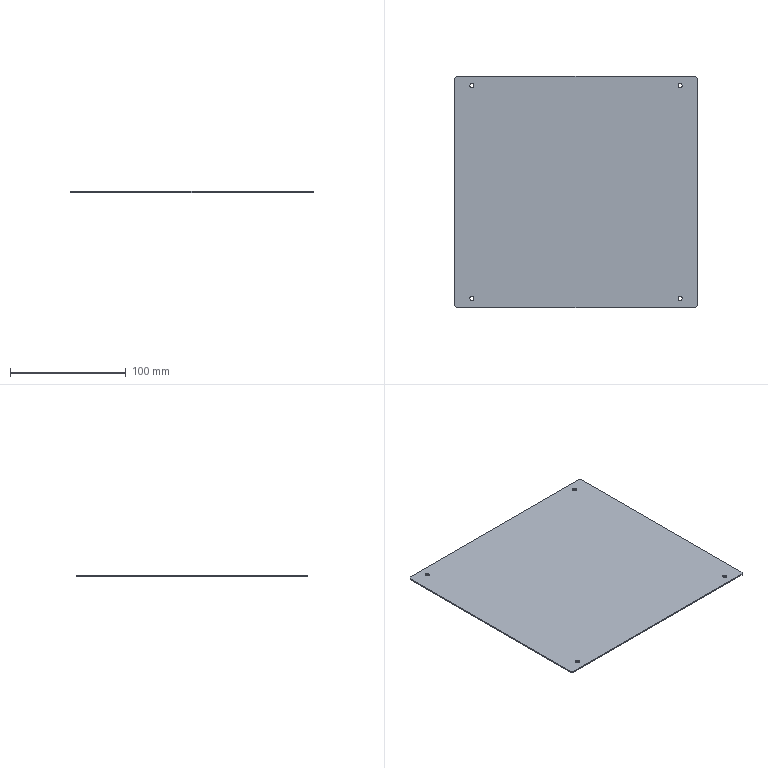Part | NX | 1 solid | 18 faces | box 210 x 200 x 1 mm | volume 41954 mm3 | plane 10 | cylinder 8 | commonest cylinder face diameters 3.5 x8
STEP:
#1=CARTESIAN_POINT('',(-105.,-98.,-0.5));
#2=VERTEX_POINT('',#1);
#3=CARTESIAN_POINT('',(-105.,98.,-0.5));
#4=VERTEX_POINT('',#3);
#5=CARTESIAN_POINT('',(-105.,-98.,-0.5));
#6=DIRECTION('',(0.,1.,0.));
#7=VECTOR('',#6,1000.);
#8=LINE('',#5,#7);
#9=EDGE_CURVE('',#2,#4,#8,.T.);
#10=ORIENTED_EDGE('',*,*,#9,.T.);
#11=CARTESIAN_POINT('',(-103.,100.,-0.5));
#12=VERTEX_POINT('',#11);
#13=CARTESIAN_POINT('',(-103.,100.,-0.5));
#14=DIRECTION('',(-0.7071,-0.7071,0.));
#15=VECTOR('',#14,1000.);
#16=LINE('',#13,#15);
#17=EDGE_CURVE('',#12,#4,#16,.T.);
#18=ORIENTED_EDGE('',*,*,#17,.F.);
#19=CARTESIAN_POINT('',(103.,100.,-0.5));
#20=VERTEX_POINT('',#19);
#21=CARTESIAN_POINT('',(-103.,100.,-0.5));
#22=DIRECTION('',(1.,0.,0.));
#23=VECTOR('',#22,1000.);
#24=LINE('',#21,#23);
#25=EDGE_CURVE('',#12,#20,#24,.T.);
#26=ORIENTED_EDGE('',*,*,#25,.T.);
#27=CARTESIAN_POINT('',(105.,98.,-0.5));
#28=VERTEX_POINT('',#27);
#29=CARTESIAN_POINT('',(105.,98.,-0.5));
#30=DIRECTION('',(-0.7071,0.7071,0.));
#31=VECTOR('',#30,1000.);
#32=LINE('',#29,#31);
#33=EDGE_CURVE('',#28,#20,#32,.T.);
#34=ORIENTED_EDGE('',*,*,#33,.F.);
#35=CARTESIAN_POINT('',(105.,-98.,-0.5));
#36=VERTEX_POINT('',#35);
#37=CARTESIAN_POINT('',(105.,98.,-0.5));
#38=DIRECTION('',(0.,-1.,0.));
#39=VECTOR('',#38,1000.);
#40=LINE('',#37,#39);
#41=EDGE_CURVE('',#28,#36,#40,.T.);
#42=ORIENTED_EDGE('',*,*,#41,.T.);
#43=CARTESIAN_POINT('',(103.,-100.,-0.5));
#44=VERTEX_POINT('',#43);
#45=CARTESIAN_POINT('',(103.,-100.,-0.5));
#46=DIRECTION('',(0.7071,0.7071,0.));
#47=VECTOR('',#46,1000.);
#48=LINE('',#45,#47);
#49=EDGE_CURVE('',#44,#36,#48,.T.);
#50=ORIENTED_EDGE('',*,*,#49,.F.);
#51=CARTESIAN_POINT('',(-103.,-100.,-0.5));
#52=VERTEX_POINT('',#51);
#53=CARTESIAN_POINT('',(103.,-100.,-0.5));
#54=DIRECTION('',(-1.,0.,0.));
#55=VECTOR('',#54,1000.);
#56=LINE('',#53,#55);
#57=EDGE_CURVE('',#44,#52,#56,.T.);
#58=ORIENTED_EDGE('',*,*,#57,.T.);
#59=CARTESIAN_POINT('',(-105.,-98.,-0.5));
#60=DIRECTION('',(0.7071,-0.7071,0.));
#61=VECTOR('',#60,1000.);
#62=LINE('',#59,#61);
#63=EDGE_CURVE('',#2,#52,#62,.T.);
#64=ORIENTED_EDGE('',*,*,#63,.F.);
#65=EDGE_LOOP('',(#10,#18,#26,#34,#42,#50,#58,#64));
#66=FACE_BOUND('',#65,.T.);
#67=CARTESIAN_POINT('',(-88.25,-92.,-0.5));
#68=VERTEX_POINT('',#67);
#69=CARTESIAN_POINT('',(-91.75,-92.,-0.5));
#70=VERTEX_POINT('',#69);
#71=CARTESIAN_POINT('',(-90.,-92.,-0.5));
#72=DIRECTION('',(0.,0.,-1.));
#73=DIRECTION('',(1.,0.,0.));
#74=AXIS2_PLACEMENT_3D('',#71,#72,#73);
#75=CIRCLE('',#74,1.75);
#76=EDGE_CURVE('',#68,#70,#75,.T.);
#77=ORIENTED_EDGE('',*,*,#76,.F.);
#78=CARTESIAN_POINT('',(-90.,-92.,-0.5));
#79=DIRECTION('',(0.,0.,-1.));
#80=DIRECTION('',(1.,0.,0.));
#81=AXIS2_PLACEMENT_3D('',#78,#79,#80);
#82=CIRCLE('',#81,1.75);
#83=EDGE_CURVE('',#70,#68,#82,.T.);
#84=ORIENTED_EDGE('',*,*,#83,.F.);
#85=EDGE_LOOP('',(#77,#84));
#86=FACE_BOUND('',#85,.T.);
#87=CARTESIAN_POINT('',(91.75,-92.,-0.5));
#88=VERTEX_POINT('',#87);
#89=CARTESIAN_POINT('',(88.25,-92.,-0.5));
#90=VERTEX_POINT('',#89);
#91=CARTESIAN_POINT('',(90.,-92.,-0.5));
#92=DIRECTION('',(0.,0.,-1.));
#93=DIRECTION('',(1.,0.,0.));
#94=AXIS2_PLACEMENT_3D('',#91,#92,#93);
#95=CIRCLE('',#94,1.75);
#96=EDGE_CURVE('',#88,#90,#95,.T.);
#97=ORIENTED_EDGE('',*,*,#96,.F.);
#98=CARTESIAN_POINT('',(90.,-92.,-0.5));
#99=DIRECTION('',(0.,0.,-1.));
#100=DIRECTION('',(1.,0.,0.));
#101=AXIS2_PLACEMENT_3D('',#98,#99,#100);
#102=CIRCLE('',#101,1.75);
#103=EDGE_CURVE('',#90,#88,#102,.T.);
#104=ORIENTED_EDGE('',*,*,#103,.F.);
#105=EDGE_LOOP('',(#97,#104));
#106=FACE_BOUND('',#105,.T.);
#107=CARTESIAN_POINT('',(-88.25,92.,-0.5));
#108=VERTEX_POINT('',#107);
#109=CARTESIAN_POINT('',(-91.75,92.,-0.5));
#110=VERTEX_POINT('',#109);
#111=CARTESIAN_POINT('',(-90.,92.,-0.5));
#112=DIRECTION('',(0.,0.,-1.));
#113=DIRECTION('',(1.,0.,0.));
#114=AXIS2_PLACEMENT_3D('',#111,#112,#113);
#115=CIRCLE('',#114,1.75);
#116=EDGE_CURVE('',#108,#110,#115,.T.);
#117=ORIENTED_EDGE('',*,*,#116,.F.);
#118=CARTESIAN_POINT('',(-90.,92.,-0.5));
#119=DIRECTION('',(0.,0.,-1.));
#120=DIRECTION('',(1.,0.,0.));
#121=AXIS2_PLACEMENT_3D('',#118,#119,#120);
#122=CIRCLE('',#121,1.75);
#123=EDGE_CURVE('',#110,#108,#122,.T.);
#124=ORIENTED_EDGE('',*,*,#123,.F.);
#125=EDGE_LOOP('',(#117,#124));
#126=FACE_BOUND('',#125,.T.);
#127=CARTESIAN_POINT('',(88.25,92.,-0.5));
#128=VERTEX_POINT('',#127);
#129=CARTESIAN_POINT('',(91.75,92.,-0.5));
#130=VERTEX_POINT('',#129);
#131=CARTESIAN_POINT('',(90.,92.,-0.5));
#132=DIRECTION('',(0.,0.,-1.));
#133=DIRECTION('',(1.,0.,0.));
#134=AXIS2_PLACEMENT_3D('',#131,#132,#133);
#135=CIRCLE('',#134,1.75);
#136=EDGE_CURVE('',#128,#130,#135,.T.);
#137=ORIENTED_EDGE('',*,*,#136,.F.);
#138=CARTESIAN_POINT('',(90.,92.,-0.5));
#139=DIRECTION('',(0.,0.,-1.));
#140=DIRECTION('',(1.,0.,0.));
#141=AXIS2_PLACEMENT_3D('',#138,#139,#140);
#142=CIRCLE('',#141,1.75);
#143=EDGE_CURVE('',#130,#128,#142,.T.);
#144=ORIENTED_EDGE('',*,*,#143,.F.);
#145=EDGE_LOOP('',(#137,#144));
#146=FACE_BOUND('',#145,.T.);
#147=CARTESIAN_POINT('',(0.,0.,-0.5));
#148=DIRECTION('',(0.,0.,1.));
#149=DIRECTION('',(1.,0.,0.));
#150=AXIS2_PLACEMENT_3D('',#147,#148,#149);
#151=PLANE('',#150);
#152=ADVANCED_FACE('',(#66,#86,#106,#126,#146),#151,.F.);
#153=ORIENTED_EDGE('',*,*,#9,.F.);
#154=CARTESIAN_POINT('',(-105.,-98.,0.5));
#155=VERTEX_POINT('',#154);
#156=CARTESIAN_POINT('',(-105.,-98.,0.5));
#157=DIRECTION('',(0.,0.,-1.));
#158=VECTOR('',#157,1000.);
#159=LINE('',#156,#158);
#160=EDGE_CURVE('',#155,#2,#159,.T.);
#161=ORIENTED_EDGE('',*,*,#160,.F.);
#162=CARTESIAN_POINT('',(-105.,98.,0.5));
#163=VERTEX_POINT('',#162);
#164=CARTESIAN_POINT('',(-105.,-98.,0.5));
#165=DIRECTION('',(0.,1.,0.));
#166=VECTOR('',#165,1000.);
#167=LINE('',#164,#166);
#168=EDGE_CURVE('',#155,#163,#167,.T.);
#169=ORIENTED_EDGE('',*,*,#168,.T.);
#170=CARTESIAN_POINT('',(-105.,98.,0.5));
#171=DIRECTION('',(0.,0.,-1.));
#172=VECTOR('',#171,1000.);
#173=LINE('',#170,#172);
#174=EDGE_CURVE('',#163,#4,#173,.T.);
#175=ORIENTED_EDGE('',*,*,#174,.T.);
#176=EDGE_LOOP('',(#153,#161,#169,#175));
#177=FACE_BOUND('',#176,.T.);
#178=CARTESIAN_POINT('',(-105.,100.,-0.5));
#179=DIRECTION('',(-1.,0.,0.));
#180=DIRECTION('',(0.,0.,1.));
#181=AXIS2_PLACEMENT_3D('',#178,#179,#180);
#182=PLANE('',#181);
#183=ADVANCED_FACE('',(#177),#182,.T.);
#184=ORIENTED_EDGE('',*,*,#174,.F.);
#185=CARTESIAN_POINT('',(-103.,100.,0.5));
#186=VERTEX_POINT('',#185);
#187=CARTESIAN_POINT('',(-105.,98.,0.5));
#188=DIRECTION('',(0.7071,0.7071,0.));
#189=VECTOR('',#188,1000.);
#190=LINE('',#187,#189);
#191=EDGE_CURVE('',#163,#186,#190,.T.);
#192=ORIENTED_EDGE('',*,*,#191,.T.);
#193=CARTESIAN_POINT('',(-103.,100.,0.5));
#194=DIRECTION('',(0.,0.,-1.));
#195=VECTOR('',#194,1000.);
#196=LINE('',#193,#195);
#197=EDGE_CURVE('',#186,#12,#196,.T.);
#198=ORIENTED_EDGE('',*,*,#197,.T.);
#199=ORIENTED_EDGE('',*,*,#17,.T.);
#200=EDGE_LOOP('',(#184,#192,#198,#199));
#201=FACE_BOUND('',#200,.T.);
#202=CARTESIAN_POINT('',(-105.,98.,-0.5));
#203=DIRECTION('',(-0.7071,0.7071,0.));
#204=DIRECTION('',(0.,0.,1.));
#205=AXIS2_PLACEMENT_3D('',#202,#203,#204);
#206=PLANE('',#205);
#207=ADVANCED_FACE('',(#201),#206,.T.);
#208=ORIENTED_EDGE('',*,*,#25,.F.);
#209=ORIENTED_EDGE('',*,*,#197,.F.);
#210=CARTESIAN_POINT('',(103.,100.,0.5));
#211=VERTEX_POINT('',#210);
#212=CARTESIAN_POINT('',(-103.,100.,0.5));
#213=DIRECTION('',(1.,0.,0.));
#214=VECTOR('',#213,1000.);
#215=LINE('',#212,#214);
#216=EDGE_CURVE('',#186,#211,#215,.T.);
#217=ORIENTED_EDGE('',*,*,#216,.T.);
#218=CARTESIAN_POINT('',(103.,100.,0.5));
#219=DIRECTION('',(0.,0.,-1.));
#220=VECTOR('',#219,1000.);
#221=LINE('',#218,#220);
#222=EDGE_CURVE('',#211,#20,#221,.T.);
#223=ORIENTED_EDGE('',*,*,#222,.T.);
#224=EDGE_LOOP('',(#208,#209,#217,#223));
#225=FACE_BOUND('',#224,.T.);
#226=CARTESIAN_POINT('',(105.,100.,-0.5));
#227=DIRECTION('',(0.,1.,0.));
#228=DIRECTION('',(1.,0.,0.));
#229=AXIS2_PLACEMENT_3D('',#226,#227,#228);
#230=PLANE('',#229);
#231=ADVANCED_FACE('',(#225),#230,.T.);
#232=ORIENTED_EDGE('',*,*,#222,.F.);
#233=CARTESIAN_POINT('',(105.,98.,0.5));
#234=VERTEX_POINT('',#233);
#235=CARTESIAN_POINT('',(103.,100.,0.5));
#236=DIRECTION('',(0.7071,-0.7071,0.));
#237=VECTOR('',#236,1000.);
#238=LINE('',#235,#237);
#239=EDGE_CURVE('',#211,#234,#238,.T.);
#240=ORIENTED_EDGE('',*,*,#239,.T.);
#241=CARTESIAN_POINT('',(105.,98.,0.5));
#242=DIRECTION('',(0.,0.,-1.));
#243=VECTOR('',#242,1000.);
#244=LINE('',#241,#243);
#245=EDGE_CURVE('',#234,#28,#244,.T.);
#246=ORIENTED_EDGE('',*,*,#245,.T.);
#247=ORIENTED_EDGE('',*,*,#33,.T.);
#248=EDGE_LOOP('',(#232,#240,#246,#247));
#249=FACE_BOUND('',#248,.T.);
#250=CARTESIAN_POINT('',(103.,100.,-0.5));
#251=DIRECTION('',(0.7071,0.7071,0.));
#252=DIRECTION('',(0.,0.,-1.));
#253=AXIS2_PLACEMENT_3D('',#250,#251,#252);
#254=PLANE('',#253);
#255=ADVANCED_FACE('',(#249),#254,.T.);
#256=ORIENTED_EDGE('',*,*,#41,.F.);
#257=ORIENTED_EDGE('',*,*,#245,.F.);
#258=CARTESIAN_POINT('',(105.,-98.,0.5));
#259=VERTEX_POINT('',#258);
#260=CARTESIAN_POINT('',(105.,98.,0.5));
#261=DIRECTION('',(0.,-1.,0.));
#262=VECTOR('',#261,1000.);
#263=LINE('',#260,#262);
#264=EDGE_CURVE('',#234,#259,#263,.T.);
#265=ORIENTED_EDGE('',*,*,#264,.T.);
#266=CARTESIAN_POINT('',(105.,-98.,0.5));
#267=DIRECTION('',(0.,0.,-1.));
#268=VECTOR('',#267,1000.);
#269=LINE('',#266,#268);
#270=EDGE_CURVE('',#259,#36,#269,.T.);
#271=ORIENTED_EDGE('',*,*,#270,.T.);
#272=EDGE_LOOP('',(#256,#257,#265,#271));
#273=FACE_BOUND('',#272,.T.);
#274=CARTESIAN_POINT('',(105.,-100.,-0.5));
#275=DIRECTION('',(1.,0.,0.));
#276=DIRECTION('',(0.,1.,0.));
#277=AXIS2_PLACEMENT_3D('',#274,#275,#276);
#278=PLANE('',#277);
#279=ADVANCED_FACE('',(#273),#278,.T.);
#280=ORIENTED_EDGE('',*,*,#270,.F.);
#281=CARTESIAN_POINT('',(103.,-100.,0.5));
#282=VERTEX_POINT('',#281);
#283=CARTESIAN_POINT('',(105.,-98.,0.5));
#284=DIRECTION('',(-0.7071,-0.7071,0.));
#285=VECTOR('',#284,1000.);
#286=LINE('',#283,#285);
#287=EDGE_CURVE('',#259,#282,#286,.T.);
#288=ORIENTED_EDGE('',*,*,#287,.T.);
#289=CARTESIAN_POINT('',(103.,-100.,0.5));
#290=DIRECTION('',(0.,0.,-1.));
#291=VECTOR('',#290,1000.);
#292=LINE('',#289,#291);
#293=EDGE_CURVE('',#282,#44,#292,.T.);
#294=ORIENTED_EDGE('',*,*,#293,.T.);
#295=ORIENTED_EDGE('',*,*,#49,.T.);
#296=EDGE_LOOP('',(#280,#288,#294,#295));
#297=FACE_BOUND('',#296,.T.);
#298=CARTESIAN_POINT('',(105.,-98.,-0.5));
#299=DIRECTION('',(0.7071,-0.7071,0.));
#300=DIRECTION('',(0.,0.,-1.));
#301=AXIS2_PLACEMENT_3D('',#298,#299,#300);
#302=PLANE('',#301);
#303=ADVANCED_FACE('',(#297),#302,.T.);
#304=ORIENTED_EDGE('',*,*,#57,.F.);
#305=ORIENTED_EDGE('',*,*,#293,.F.);
#306=CARTESIAN_POINT('',(-103.,-100.,0.5));
#307=VERTEX_POINT('',#306);
#308=CARTESIAN_POINT('',(103.,-100.,0.5));
#309=DIRECTION('',(-1.,0.,0.));
#310=VECTOR('',#309,1000.);
#311=LINE('',#308,#310);
#312=EDGE_CURVE('',#282,#307,#311,.T.);
#313=ORIENTED_EDGE('',*,*,#312,.T.);
#314=CARTESIAN_POINT('',(-103.,-100.,0.5));
#315=DIRECTION('',(0.,0.,-1.));
#316=VECTOR('',#315,1000.);
#317=LINE('',#314,#316);
#318=EDGE_CURVE('',#307,#52,#317,.T.);
#319=ORIENTED_EDGE('',*,*,#318,.T.);
#320=EDGE_LOOP('',(#304,#305,#313,#319));
#321=FACE_BOUND('',#320,.T.);
#322=CARTESIAN_POINT('',(-105.,-100.,-0.5));
#323=DIRECTION('',(0.,-1.,0.));
#324=DIRECTION('',(0.,0.,-1.));
#325=AXIS2_PLACEMENT_3D('',#322,#323,#324);
#326=PLANE('',#325);
#327=ADVANCED_FACE('',(#321),#326,.T.);
#328=ORIENTED_EDGE('',*,*,#318,.F.);
#329=CARTESIAN_POINT('',(-103.,-100.,0.5));
#330=DIRECTION('',(-0.7071,0.7071,0.));
#331=VECTOR('',#330,1000.);
#332=LINE('',#329,#331);
#333=EDGE_CURVE('',#307,#155,#332,.T.);
#334=ORIENTED_EDGE('',*,*,#333,.T.);
#335=ORIENTED_EDGE('',*,*,#160,.T.);
#336=ORIENTED_EDGE('',*,*,#63,.T.);
#337=EDGE_LOOP('',(#328,#334,#335,#336));
#338=FACE_BOUND('',#337,.T.);
#339=CARTESIAN_POINT('',(-103.,-100.,-0.5));
#340=DIRECTION('',(-0.7071,-0.7071,0.));
#341=DIRECTION('',(-0.7071,0.7071,0.));
#342=AXIS2_PLACEMENT_3D('',#339,#340,#341);
#343=PLANE('',#342);
#344=ADVANCED_FACE('',(#338),#343,.T.);
#345=ORIENTED_EDGE('',*,*,#168,.F.);
#346=ORIENTED_EDGE('',*,*,#333,.F.);
#347=ORIENTED_EDGE('',*,*,#312,.F.);
#348=ORIENTED_EDGE('',*,*,#287,.F.);
#349=ORIENTED_EDGE('',*,*,#264,.F.);
#350=ORIENTED_EDGE('',*,*,#239,.F.);
#351=ORIENTED_EDGE('',*,*,#216,.F.);
#352=ORIENTED_EDGE('',*,*,#191,.F.);
#353=EDGE_LOOP('',(#345,#346,#347,#348,#349,#350,#351,#352));
#354=FACE_BOUND('',#353,.T.);
#355=CARTESIAN_POINT('',(-88.25,-92.,0.5));
#356=VERTEX_POINT('',#355);
#357=CARTESIAN_POINT('',(-91.75,-92.,0.5));
#358=VERTEX_POINT('',#357);
#359=CARTESIAN_POINT('',(-90.,-92.,0.5));
#360=DIRECTION('',(0.,0.,1.));
#361=DIRECTION('',(-1.,0.,0.));
#362=AXIS2_PLACEMENT_3D('',#359,#360,#361);
#363=CIRCLE('',#362,1.75);
#364=EDGE_CURVE('',#356,#358,#363,.T.);
#365=ORIENTED_EDGE('',*,*,#364,.F.);
#366=CARTESIAN_POINT('',(-90.,-92.,0.5));
#367=DIRECTION('',(0.,0.,1.));
#368=DIRECTION('',(-1.,0.,0.));
#369=AXIS2_PLACEMENT_3D('',#366,#367,#368);
#370=CIRCLE('',#369,1.75);
#371=EDGE_CURVE('',#358,#356,#370,.T.);
#372=ORIENTED_EDGE('',*,*,#371,.F.);
#373=EDGE_LOOP('',(#365,#372));
#374=FACE_BOUND('',#373,.T.);
#375=CARTESIAN_POINT('',(88.25,-92.,0.5));
#376=VERTEX_POINT('',#375);
#377=CARTESIAN_POINT('',(91.75,-92.,0.5));
#378=VERTEX_POINT('',#377);
#379=CARTESIAN_POINT('',(90.,-92.,0.5));
#380=DIRECTION('',(0.,0.,1.));
#381=DIRECTION('',(-1.,0.,0.));
#382=AXIS2_PLACEMENT_3D('',#379,#380,#381);
#383=CIRCLE('',#382,1.75);
#384=EDGE_CURVE('',#376,#378,#383,.T.);
#385=ORIENTED_EDGE('',*,*,#384,.F.);
#386=CARTESIAN_POINT('',(90.,-92.,0.5));
#387=DIRECTION('',(0.,0.,1.));
#388=DIRECTION('',(-1.,0.,0.));
#389=AXIS2_PLACEMENT_3D('',#386,#387,#388);
#390=CIRCLE('',#389,1.75);
#391=EDGE_CURVE('',#378,#376,#390,.T.);
#392=ORIENTED_EDGE('',*,*,#391,.F.);
#393=EDGE_LOOP('',(#385,#392));
#394=FACE_BOUND('',#393,.T.);
#395=CARTESIAN_POINT('',(-88.25,92.,0.5));
#396=VERTEX_POINT('',#395);
#397=CARTESIAN_POINT('',(-91.75,92.,0.5));
#398=VERTEX_POINT('',#397);
#399=CARTESIAN_POINT('',(-90.,92.,0.5));
#400=DIRECTION('',(0.,0.,1.));
#401=DIRECTION('',(-1.,0.,0.));
#402=AXIS2_PLACEMENT_3D('',#399,#400,#401);
#403=CIRCLE('',#402,1.75);
#404=EDGE_CURVE('',#396,#398,#403,.T.);
#405=ORIENTED_EDGE('',*,*,#404,.F.);
#406=CARTESIAN_POINT('',(-90.,92.,0.5));
#407=DIRECTION('',(0.,0.,1.));
#408=DIRECTION('',(-1.,0.,0.));
#409=AXIS2_PLACEMENT_3D('',#406,#407,#408);
#410=CIRCLE('',#409,1.75);
#411=EDGE_CURVE('',#398,#396,#410,.T.);
#412=ORIENTED_EDGE('',*,*,#411,.F.);
#413=EDGE_LOOP('',(#405,#412));
#414=FACE_BOUND('',#413,.T.);
#415=CARTESIAN_POINT('',(91.75,92.,0.5));
#416=VERTEX_POINT('',#415);
#417=CARTESIAN_POINT('',(88.25,92.,0.5));
#418=VERTEX_POINT('',#417);
#419=CARTESIAN_POINT('',(90.,92.,0.5));
#420=DIRECTION('',(0.,0.,1.));
#421=DIRECTION('',(-1.,0.,0.));
#422=AXIS2_PLACEMENT_3D('',#419,#420,#421);
#423=CIRCLE('',#422,1.75);
#424=EDGE_CURVE('',#416,#418,#423,.T.);
#425=ORIENTED_EDGE('',*,*,#424,.F.);
#426=CARTESIAN_POINT('',(90.,92.,0.5));
#427=DIRECTION('',(0.,0.,1.));
#428=DIRECTION('',(-1.,0.,0.));
#429=AXIS2_PLACEMENT_3D('',#426,#427,#428);
#430=CIRCLE('',#429,1.75);
#431=EDGE_CURVE('',#418,#416,#430,.T.);
#432=ORIENTED_EDGE('',*,*,#431,.F.);
#433=EDGE_LOOP('',(#425,#432));
#434=FACE_BOUND('',#433,.T.);
#435=CARTESIAN_POINT('',(0.,0.,0.5));
#436=DIRECTION('',(0.,0.,1.));
#437=DIRECTION('',(1.,0.,0.));
#438=AXIS2_PLACEMENT_3D('',#435,#436,#437);
#439=PLANE('',#438);
#440=ADVANCED_FACE('',(#354,#374,#394,#414,#434),#439,.T.);
#441=ORIENTED_EDGE('',*,*,#364,.T.);
#442=CARTESIAN_POINT('',(-91.75,-92.,0.5));
#443=DIRECTION('',(0.,0.,-1.));
#444=VECTOR('',#443,1000.);
#445=LINE('',#442,#444);
#446=EDGE_CURVE('',#70,#358,#445,.F.);
#447=ORIENTED_EDGE('',*,*,#446,.F.);
#448=ORIENTED_EDGE('',*,*,#83,.T.);
#449=CARTESIAN_POINT('',(-88.25,-92.,0.5));
#450=DIRECTION('',(0.,0.,-1.));
#451=VECTOR('',#450,1000.);
#452=LINE('',#449,#451);
#453=EDGE_CURVE('',#68,#356,#452,.F.);
#454=ORIENTED_EDGE('',*,*,#453,.T.);
#455=EDGE_LOOP('',(#441,#447,#448,#454));
#456=FACE_BOUND('',#455,.T.);
#457=CARTESIAN_POINT('',(-90.,-92.,0.5));
#458=DIRECTION('',(0.,0.,-1.));
#459=DIRECTION('',(-1.,0.,0.));
#460=AXIS2_PLACEMENT_3D('',#457,#458,#459);
#461=CYLINDRICAL_SURFACE('',#460,1.75);
#462=ADVANCED_FACE('',(#456),#461,.F.);
#463=ORIENTED_EDGE('',*,*,#404,.T.);
#464=CARTESIAN_POINT('',(-91.75,92.,0.5));
#465=DIRECTION('',(0.,0.,-1.));
#466=VECTOR('',#465,1000.);
#467=LINE('',#464,#466);
#468=EDGE_CURVE('',#110,#398,#467,.F.);
#469=ORIENTED_EDGE('',*,*,#468,.F.);
#470=ORIENTED_EDGE('',*,*,#123,.T.);
#471=CARTESIAN_POINT('',(-88.25,92.,0.5));
#472=DIRECTION('',(0.,0.,-1.));
#473=VECTOR('',#472,1000.);
#474=LINE('',#471,#473);
#475=EDGE_CURVE('',#108,#396,#474,.F.);
#476=ORIENTED_EDGE('',*,*,#475,.T.);
#477=EDGE_LOOP('',(#463,#469,#470,#476));
#478=FACE_BOUND('',#477,.T.);
#479=CARTESIAN_POINT('',(-90.,92.,0.5));
#480=DIRECTION('',(0.,0.,-1.));
#481=DIRECTION('',(-1.,0.,0.));
#482=AXIS2_PLACEMENT_3D('',#479,#480,#481);
#483=CYLINDRICAL_SURFACE('',#482,1.75);
#484=ADVANCED_FACE('',(#478),#483,.F.);
#485=ORIENTED_EDGE('',*,*,#96,.T.);
#486=CARTESIAN_POINT('',(88.25,-92.,0.5));
#487=DIRECTION('',(0.,0.,-1.));
#488=VECTOR('',#487,1000.);
#489=LINE('',#486,#488);
#490=EDGE_CURVE('',#90,#376,#489,.F.);
#491=ORIENTED_EDGE('',*,*,#490,.T.);
#492=ORIENTED_EDGE('',*,*,#384,.T.);
#493=CARTESIAN_POINT('',(91.75,-92.,0.5));
#494=DIRECTION('',(0.,0.,-1.));
#495=VECTOR('',#494,1000.);
#496=LINE('',#493,#495);
#497=EDGE_CURVE('',#88,#378,#496,.F.);
#498=ORIENTED_EDGE('',*,*,#497,.F.);
#499=EDGE_LOOP('',(#485,#491,#492,#498));
#500=FACE_BOUND('',#499,.T.);
#501=CARTESIAN_POINT('',(90.,-92.,0.5));
#502=DIRECTION('',(0.,0.,-1.));
#503=DIRECTION('',(-1.,0.,0.));
#504=AXIS2_PLACEMENT_3D('',#501,#502,#503);
#505=CYLINDRICAL_SURFACE('',#504,1.75);
#506=ADVANCED_FACE('',(#500),#505,.F.);
#507=ORIENTED_EDGE('',*,*,#136,.T.);
#508=CARTESIAN_POINT('',(91.75,92.,0.5));
#509=DIRECTION('',(0.,0.,-1.));
#510=VECTOR('',#509,1000.);
#511=LINE('',#508,#510);
#512=EDGE_CURVE('',#130,#416,#511,.F.);
#513=ORIENTED_EDGE('',*,*,#512,.T.);
#514=ORIENTED_EDGE('',*,*,#424,.T.);
#515=CARTESIAN_POINT('',(88.25,92.,0.5));
#516=DIRECTION('',(0.,0.,-1.));
#517=VECTOR('',#516,1000.);
#518=LINE('',#515,#517);
#519=EDGE_CURVE('',#128,#418,#518,.F.);
#520=ORIENTED_EDGE('',*,*,#519,.F.);
#521=EDGE_LOOP('',(#507,#513,#514,#520));
#522=FACE_BOUND('',#521,.T.);
#523=CARTESIAN_POINT('',(90.,92.,0.5));
#524=DIRECTION('',(0.,0.,-1.));
#525=DIRECTION('',(-1.,0.,0.));
#526=AXIS2_PLACEMENT_3D('',#523,#524,#525);
#527=CYLINDRICAL_SURFACE('',#526,1.75);
#528=ADVANCED_FACE('',(#522),#527,.F.);
#529=ORIENTED_EDGE('',*,*,#519,.T.);
#530=ORIENTED_EDGE('',*,*,#431,.T.);
#531=ORIENTED_EDGE('',*,*,#512,.F.);
#532=ORIENTED_EDGE('',*,*,#143,.T.);
#533=EDGE_LOOP('',(#529,#530,#531,#532));
#534=FACE_BOUND('',#533,.T.);
#535=CARTESIAN_POINT('',(90.,92.,0.5));
#536=DIRECTION('',(0.,0.,-1.));
#537=DIRECTION('',(-1.,0.,0.));
#538=AXIS2_PLACEMENT_3D('',#535,#536,#537);
#539=CYLINDRICAL_SURFACE('',#538,1.75);
#540=ADVANCED_FACE('',(#534),#539,.F.);
#541=ORIENTED_EDGE('',*,*,#116,.T.);
#542=ORIENTED_EDGE('',*,*,#468,.T.);
#543=ORIENTED_EDGE('',*,*,#411,.T.);
#544=ORIENTED_EDGE('',*,*,#475,.F.);
#545=EDGE_LOOP('',(#541,#542,#543,#544));
#546=FACE_BOUND('',#545,.T.);
#547=CARTESIAN_POINT('',(-90.,92.,0.5));
#548=DIRECTION('',(0.,0.,-1.));
#549=DIRECTION('',(-1.,0.,0.));
#550=AXIS2_PLACEMENT_3D('',#547,#548,#549);
#551=CYLINDRICAL_SURFACE('',#550,1.75);
#552=ADVANCED_FACE('',(#546),#551,.F.);
#553=ORIENTED_EDGE('',*,*,#490,.F.);
#554=ORIENTED_EDGE('',*,*,#103,.T.);
#555=ORIENTED_EDGE('',*,*,#497,.T.);
#556=ORIENTED_EDGE('',*,*,#391,.T.);
#557=EDGE_LOOP('',(#553,#554,#555,#556));
#558=FACE_BOUND('',#557,.T.);
#559=CARTESIAN_POINT('',(90.,-92.,0.5));
#560=DIRECTION('',(0.,0.,-1.));
#561=DIRECTION('',(-1.,0.,0.));
#562=AXIS2_PLACEMENT_3D('',#559,#560,#561);
#563=CYLINDRICAL_SURFACE('',#562,1.75);
#564=ADVANCED_FACE('',(#558),#563,.F.);
#565=ORIENTED_EDGE('',*,*,#76,.T.);
#566=ORIENTED_EDGE('',*,*,#446,.T.);
#567=ORIENTED_EDGE('',*,*,#371,.T.);
#568=ORIENTED_EDGE('',*,*,#453,.F.);
#569=EDGE_LOOP('',(#565,#566,#567,#568));
#570=FACE_BOUND('',#569,.T.);
#571=CARTESIAN_POINT('',(-90.,-92.,0.5));
#572=DIRECTION('',(0.,0.,-1.));
#573=DIRECTION('',(-1.,0.,0.));
#574=AXIS2_PLACEMENT_3D('',#571,#572,#573);
#575=CYLINDRICAL_SURFACE('',#574,1.75);
#576=ADVANCED_FACE('',(#570),#575,.F.);
#577=CLOSED_SHELL('',(#152,#183,#207,#231,#255,#279,#303,#327,#344,#440,#462,#484,#506,#528,#540,#552,#564,#576));
#578=MANIFOLD_SOLID_BREP('',#577);
#579=(LENGTH_UNIT()NAMED_UNIT(*)SI_UNIT(.MILLI.,.METRE.));
#580=UNCERTAINTY_MEASURE_WITH_UNIT(LENGTH_MEASURE(0.00001),#579,'','');
#581=(NAMED_UNIT(*)PLANE_ANGLE_UNIT()SI_UNIT($,.RADIAN.));
#582=(NAMED_UNIT(*)SI_UNIT($,.STERADIAN.)SOLID_ANGLE_UNIT());
#583=(GEOMETRIC_REPRESENTATION_CONTEXT(3)GLOBAL_UNCERTAINTY_ASSIGNED_CONTEXT((#580))GLOBAL_UNIT_ASSIGNED_CONTEXT((#579,#581,#582))REPRESENTATION_CONTEXT('',''));
#584=ADVANCED_BREP_SHAPE_REPRESENTATION('',(#578),#583);